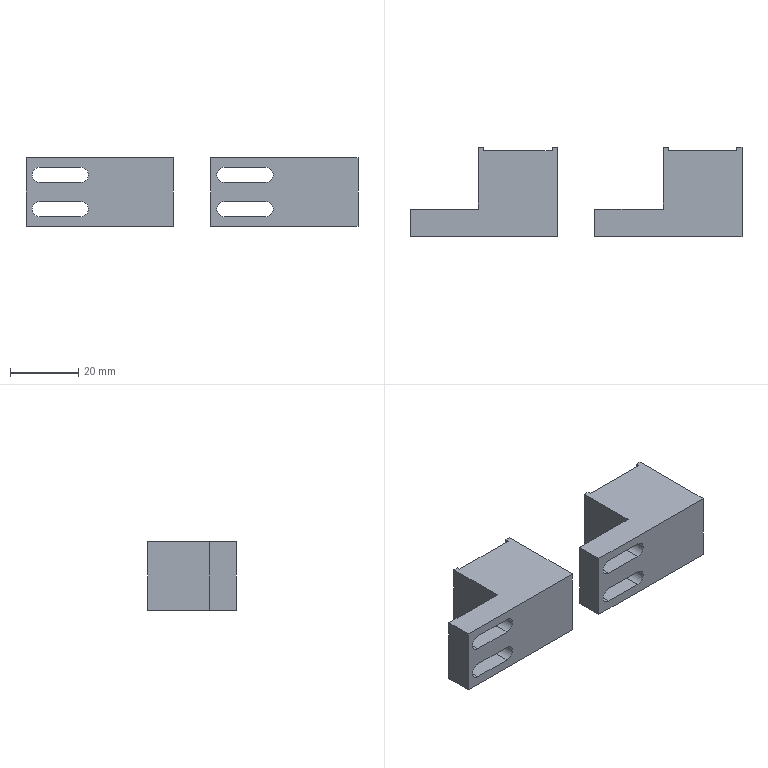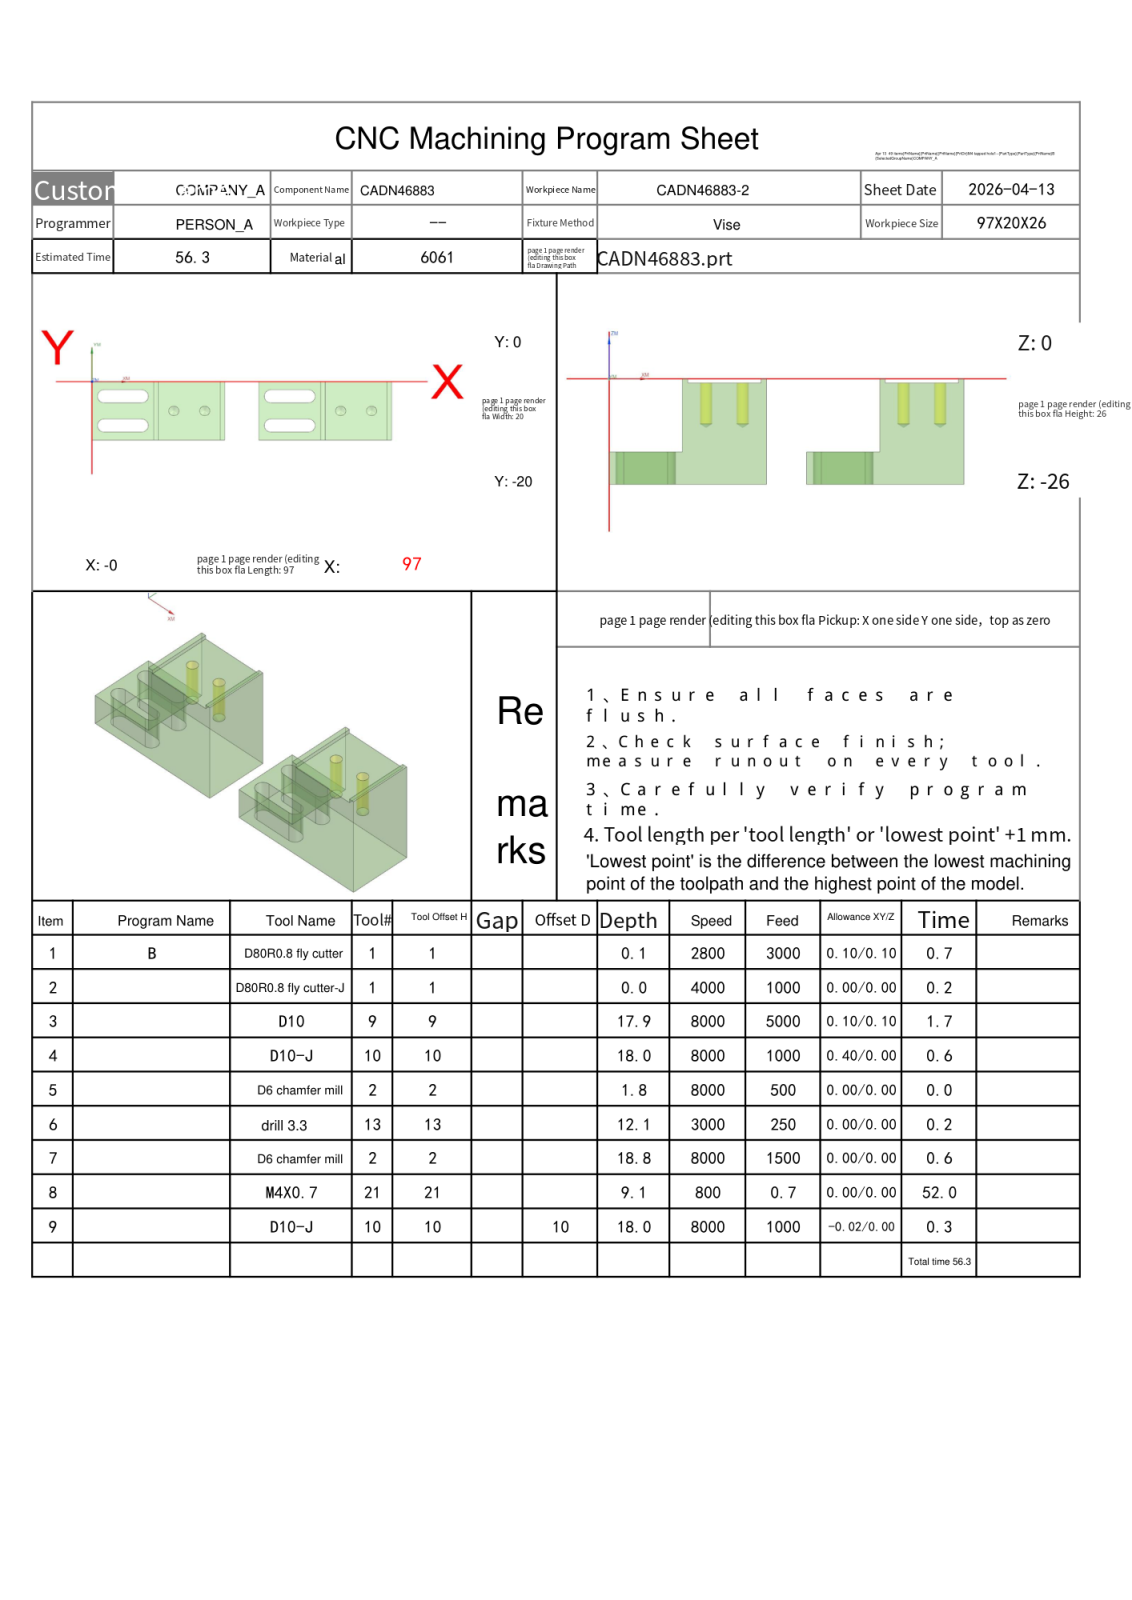NC program | NX | posted by the shop | part box 97 x 26 x 20 mm
Whole program:
%
O0001
(Machine time: 104.35 MIN)
(===Total Tool:6===)
(T1=D80R0.8 fly cutter D=80.  R=0.8  D-  H01 Z=-0.   )
(T9=D10     D=10.  R=0.   D-  H09 Z=-17.9 )
(T10=D10-J  D=10.  R=0.   D-  H10 Z=-18.  )
(T2=D6 chamfer mill   D=6.   R=0.   D-  H02 Z=-18.8 )
(T13=drill 3.3  D=3.3  DR_a=118 D-  H13 Z=-12.09)
(T21=M4X0.7 D=3.3  DR_a=180 D-  H21 Z=-9.1  )
G80 G90 G17 G49 G40
G91 G28 Z0
M01
N1 T01 M06
(D80R0.8 fly cutter  D=80. R=0.8 H=01 ce=0.10 di=0.10)
G00 G90 G54 X149.097 Y-10. M03 S2800
G43 H01 Z20.
M08
Z5.513
G01 Z3.513 F3000.
X137.097
X-40.097
X-52.097
Z5.513
G00 X149.097
Z5.025
G01 Z3.025
X137.097
X-40.097
X-52.097
Z5.025
G00 X149.097
Z4.538
G01 Z2.538
X137.097
X-40.097
X-52.097
Z4.538
G00 X149.097
Z4.05
G01 Z2.05
X137.097
X-40.097
X-52.097
Z4.05
G00 Z20.
X149.097
Z3.563
G01 Z1.563
X137.097
X-40.097
X-52.097
Z3.563
G00 Z20.
X149.097
Z3.075
G01 Z1.075
X137.097
X-40.097
X-52.097
Z3.075
G00 Z20.
X149.097
Z2.588
G01 Z.588
X137.097
X-40.097
X-52.097
Z2.588
G00 Z20.
X149.097
Z2.1
G01 Z.1
X137.097
X-40.097
X-52.097
Z2.1
G00 Z20.
G91 G28 Z0.0
M05
M09
G91 G28 Z0.0
M01
N2 T01 M06
(D80R0.8 fly cutter-J  D=80. R=0.8 H=01 ce=0.00 di=0.00)
G00 G90 G54 X148.999 Y-10. M03 S4000
G43 H01 Z20.
M08
Z2.
G01 Z0.0 F1000.
X136.999
X-39.999
X-51.999
Z2.
G00 Z20.
G91 G28 Z0.0
M05
M09
G91 G28 Z0.0
M01
N3 T09 M06
(D10  D=10. R=0. H=09 ce=0.10 di=0.10)
G00 G90 G54 X-.1 Y-28. M03 S8000
G43 H09 Z13.8
M08
Z.903
G01 Z-.597 F5000.
Y-24.9
Y3.9
G02 X.9 Y4.9 I1. J0.0
G01 X6.4
G02 X7.4 Y3.9 I0.0 J-1.
G01 Y-24.044
G03 X8.246 Y-25.032 I1. J0.0
G01 X13.746 Y-25.888
X13.9 Y-25.9
G03 X14.9 Y-24.9 I0.0 J1.
G01 Y4.9
Y8.1
Z.903
G00 X-.1 Y-28.
Z.307
G01 Z-1.193
Y-24.9
Y3.9
G02 X.9 Y4.9 I1. J0.0
G01 X6.4
G02 X7.4 Y3.9 I0.0 J-1.
G01 Y-24.044
G03 X8.246 Y-25.032 I1. J0.0
G01 X13.746 Y-25.888
X13.9 Y-25.9
G03 X14.9 Y-24.9 I0.0 J1.
G01 Y4.9
Y8.1
Z.307
G00 X-.1 Y-28.
Z-.29
G01 Z-1.79
Y-24.9
Y3.9
G02 X.9 Y4.9 I1. J0.0
G01 X6.4
G02 X7.4 Y3.9 I0.0 J-1.
G01 Y-24.044
G03 X8.246 Y-25.032 I1. J0.0
G01 X13.746 Y-25.888
X13.9 Y-25.9
G03 X14.9 Y-24.9 I0.0 J1.
G01 Y4.9
Y8.1
Z-.29
G00 X-.1 Y-28.
Z-.887
G01 Z-2.387
Y-24.9
Y3.9
G02 X.9 Y4.9 I1. J0.0
G01 X6.4
G02 X7.4 Y3.9 I0.0 J-1.
G01 Y-24.044
G03 X8.246 Y-25.032 I1. J0.0
G01 X13.746 Y-25.888
X13.9 Y-25.9
G03 X14.9 Y-24.9 I0.0 J1.
G01 Y4.9
Y8.1
Z-.887
G00 X-.1 Y-28.
Z-1.483
G01 Z-2.983
Y-24.9
Y3.9
G02 X.9 Y4.9 I1. J0.0
G01 X6.4
G02 X7.4 Y3.9 I0.0 J-1.
G01 Y-24.044
G03 X8.246 Y-25.032 I1. J0.0
G01 X13.746 Y-25.888
X13.9 Y-25.9
G03 X14.9 Y-24.9 I0.0 J1.
G01 Y4.9
Y8.1
Z-1.483
G00 X-.1 Y-28.
Z-2.08
G01 Z-3.58
Y-24.9
Y3.9
G02 X.9 Y4.9 I1. J0.0
G01 X6.4
G02 X7.4 Y3.9 I0.0 J-1.
G01 Y-24.044
G03 X8.246 Y-25.032 I1. J0.0
G01 X13.746 Y-25.888
X13.9 Y-25.9
G03 X14.9 Y-24.9 I0.0 J1.
G01 Y4.9
Y8.1
Z-2.08
G00 X-.1 Y-28.
Z-2.677
G01 Z-4.177
Y-24.9
Y3.9
G02 X.9 Y4.9 I1. J0.0
G01 X6.4
G02 X7.4 Y3.9 I0.0 J-1.
G01 Y-24.044
G03 X8.246 Y-25.032 I1. J0.0
G01 X13.746 Y-25.888
X13.9 Y-25.9
G03 X14.9 Y-24.9 I0.0 J1.
G01 Y4.9
Y8.1
Z-2.677
G00 X-.1 Y-28.
Z-3.273
G01 Z-4.773
Y-24.9
Y3.9
G02 X.9 Y4.9 I1. J0.0
G01 X6.4
G02 X7.4 Y3.9 I0.0 J-1.
G01 Y-24.044
G03 X8.246 Y-25.032 I1. J0.0
G01 X13.746 Y-25.888
X13.9 Y-25.9
G03 X14.9 Y-24.9 I0.0 J1.
G01 Y4.9
Y8.1
Z-3.273
G00 X-.1 Y-28.
Z-3.87
G01 Z-5.37
Y-24.9
Y3.9
G02 X.9 Y4.9 I1. J0.0
G01 X6.4
G02 X7.4 Y3.9 I0.0 J-1.
G01 Y-24.044
G03 X8.246 Y-25.032 I1. J0.0
G01 X13.746 Y-25.888
X13.9 Y-25.9
G03 X14.9 Y-24.9 I0.0 J1.
G01 Y4.9
Y8.1
Z-3.87
G00 X-.1 Y-28.
Z-4.467
G01 Z-5.967
Y-24.9
Y3.9
G02 X.9 Y4.9 I1. J0.0
G01 X6.4
G02 X7.4 Y3.9 I0.0 J-1.
G01 Y-24.044
G03 X8.246 Y-25.032 I1. J0.0
G01 X13.746 Y-25.888
X13.9 Y-25.9
G03 X14.9 Y-24.9 I0.0 J1.
G01 Y4.9
Y8.1
Z-4.467
G00 X-.1 Y-28.
Z-5.063
G01 Z-6.563
Y-24.9
Y3.9
G02 X.9 Y4.9 I1. J0.0
G01 X6.4
G02 X7.4 Y3.9 I0.0 J-1.
G01 Y-24.044
G03 X8.246 Y-25.032 I1. J0.0
G01 X13.746 Y-25.888
X13.9 Y-25.9
G03 X14.9 Y-24.9 I0.0 J1.
G01 Y4.9
Y8.1
Z-5.063
G00 X-.1 Y-28.
Z-5.66
G01 Z-7.16
Y-24.9
Y3.9
G02 X.9 Y4.9 I1. J0.0
G01 X6.4
G02 X7.4 Y3.9 I0.0 J-1.
G01 Y-24.044
G03 X8.246 Y-25.032 I1. J0.0
G01 X13.746 Y-25.888
X13.9 Y-25.9
G03 X14.9 Y-24.9 I0.0 J1.
G01 Y4.9
Y8.1
Z-5.66
G00 X-.1 Y-28.
Z-6.257
G01 Z-7.757
Y-24.9
Y3.9
G02 X.9 Y4.9 I1. J0.0
G01 X6.4
G02 X7.4 Y3.9 I0.0 J-1.
G01 Y-24.044
G03 X8.246 Y-25.032 I1. J0.0
G01 X13.746 Y-25.888
X13.9 Y-25.9
G03 X14.9 Y-24.9 I0.0 J1.
G01 Y4.9
Y8.1
Z-6.257
G00 X-.1 Y-28.
Z-6.853
G01 Z-8.353
Y-24.9
Y3.9
G02 X.9 Y4.9 I1. J0.0
G01 X6.4
G02 X7.4 Y3.9 I0.0 J-1.
G01 Y-24.044
G03 X8.246 Y-25.032 I1. J0.0
G01 X13.746 Y-25.888
X13.9 Y-25.9
G03 X14.9 Y-24.9 I0.0 J1.
G01 Y4.9
Y8.1
Z-6.853
G00 X-.1 Y-28.
Z-7.45
G01 Z-8.95
Y-24.9
Y3.9
G02 X.9 Y4.9 I1. J0.0
G01 X6.4
G02 X7.4 Y3.9 I0.0 J-1.
G01 Y-24.044
G03 X8.246 Y-25.032 I1. J0.0
G01 X13.746 Y-25.888
X13.9 Y-25.9
G03 X14.9 Y-24.9 I0.0 J1.
G01 Y4.9
Y8.1
Z-7.45
G00 X-.1 Y-28.
Z-8.047
G01 Z-9.547
Y-24.9
Y3.9
G02 X.9 Y4.9 I1. J0.0
G01 X6.4
G02 X7.4 Y3.9 I0.0 J-1.
G01 Y-24.044
G03 X8.246 Y-25.032 I1. J0.0
G01 X13.746 Y-25.888
X13.9 Y-25.9
G03 X14.9 Y-24.9 I0.0 J1.
G01 Y4.9
Y8.1
Z-8.047
G00 X-.1 Y-28.
Z-8.643
G01 Z-10.143
Y-24.9
Y3.9
G02 X.9 Y4.9 I1. J0.0
G01 X6.4
G02 X7.4 Y3.9 I0.0 J-1.
G01 Y-24.044
G03 X8.246 Y-25.032 I1. J0.0
G01 X13.746 Y-25.888
X13.9 Y-25.9
G03 X14.9 Y-24.9 I0.0 J1.
G01 Y4.9
Y8.1
Z-8.643
G00 X-.1 Y-28.
Z-9.24
G01 Z-10.74
Y-24.9
Y3.9
G02 X.9 Y4.9 I1. J0.0
G01 X6.4
G02 X7.4 Y3.9 I0.0 J-1.
G01 Y-24.044
G03 X8.246 Y-25.032 I1. J0.0
G01 X13.746 Y-25.888
X13.9 Y-25.9
G03 X14.9 Y-24.9 I0.0 J1.
G01 Y4.9
Y8.1
Z-9.24
G00 X-.1 Y-28.
Z-9.837
G01 Z-11.337
Y-24.9
Y3.9
G02 X.9 Y4.9 I1. J0.0
G01 X6.4
G02 X7.4 Y3.9 I0.0 J-1.
G01 Y-24.044
G03 X8.246 Y-25.032 I1. J0.0
G01 X13.746 Y-25.888
X13.9 Y-25.9
G03 X14.9 Y-24.9 I0.0 J1.
G01 Y4.9
Y8.1
Z-9.837
G00 X-.1 Y-28.
Z-10.433
G01 Z-11.933
Y-24.9
Y3.9
G02 X.9 Y4.9 I1. J0.0
G01 X6.4
G02 X7.4 Y3.9 I0.0 J-1.
G01 Y-24.044
G03 X8.246 Y-25.032 I1. J0.0
G01 X13.746 Y-25.888
X13.9 Y-25.9
G03 X14.9 Y-24.9 I0.0 J1.
G01 Y4.9
Y8.1
Z-10.433
G00 X-.1 Y-28.
Z-11.03
G01 Z-12.53
Y-24.9
Y3.9
G02 X.9 Y4.9 I1. J0.0
G01 X6.4
G02 X7.4 Y3.9 I0.0 J-1.
G01 Y-24.044
G03 X8.246 Y-25.032 I1. J0.0
G01 X13.746 Y-25.888
X13.9 Y-25.9
G03 X14.9 Y-24.9 I0.0 J1.
G01 Y4.9
Y8.1
Z-11.03
G00 X-.1 Y-28.
Z-11.627
G01 Z-13.127
Y-24.9
Y3.9
G02 X.9 Y4.9 I1. J0.0
G01 X6.4
G02 X7.4 Y3.9 I0.0 J-1.
G01 Y-24.044
G03 X8.246 Y-25.032 I1. J0.0
G01 X13.746 Y-25.888
X13.9 Y-25.9
G03 X14.9 Y-24.9 I0.0 J1.
G01 Y4.9
Y8.1
Z-11.627
G00 X-.1 Y-28.
Z-12.223
G01 Z-13.723
Y-24.9
Y3.9
G02 X.9 Y4.9 I1. J0.0
G01 X6.4
G02 X7.4 Y3.9 I0.0 J-1.
G01 Y-24.044
G03 X8.246 Y-25.032 I1. J0.0
G01 X13.746 Y-25.888
X13.9 Y-25.9
G03 X14.9 Y-24.9 I0.0 J1.
G01 Y4.9
Y8.1
Z-12.223
G00 X-.1 Y-28.
Z-12.82
G01 Z-14.32
Y-24.9
Y3.9
G02 X.9 Y4.9 I1. J0.0
G01 X6.4
G02 X7.4 Y3.9 I0.0 J-1.
G01 Y-24.044
G03 X8.246 Y-25.032 I1. J0.0
G01 X13.746 Y-25.888
X13.9 Y-25.9
G03 X14.9 Y-24.9 I0.0 J1.
G01 Y4.9
Y8.1
Z-12.82
G00 X-.1 Y-28.
Z-13.417
G01 Z-14.917
Y-24.9
Y3.9
G02 X.9 Y4.9 I1. J0.0
G01 X6.4
G02 X7.4 Y3.9 I0.0 J-1.
G01 Y-24.044
G03 X8.246 Y-25.032 I1. J0.0
G01 X13.746 Y-25.888
X13.9 Y-25.9
G03 X14.9 Y-24.9 I0.0 J1.
G01 Y4.9
Y8.1
Z-13.417
G00 X-.1 Y-28.
Z-14.013
G01 Z-15.513
Y-24.9
Y3.9
G02 X.9 Y4.9 I1. J0.0
G01 X6.4
G02 X7.4 Y3.9 I0.0 J-1.
G01 Y-24.044
G03 X8.246 Y-25.032 I1. J0.0
G01 X13.746 Y-25.888
X13.9 Y-25.9
G03 X14.9 Y-24.9 I0.0 J1.
G01 Y4.9
Y8.1
Z-14.013
G00 X-.1 Y-28.
Z-14.61
G01 Z-16.11
Y-24.9
Y3.9
G02 X.9 Y4.9 I1. J0.0
G01 X6.4
G02 X7.4 Y3.9 I0.0 J-1.
G01 Y-24.044
G03 X8.246 Y-25.032 I1. J0.0
G01 X13.746 Y-25.888
X13.9 Y-25.9
G03 X14.9 Y-24.9 I0.0 J1.
G01 Y4.9
Y8.1
Z-14.61
G00 X-.1 Y-28.
Z-15.207
G01 Z-16.707
Y-24.9
Y3.9
G02 X.9 Y4.9 I1. J0.0
G01 X6.4
G02 X7.4 Y3.9 I0.0 J-1.
G01 Y-24.044
G03 X8.246 Y-25.032 I1. J0.0
G01 X13.746 Y-25.888
X13.9 Y-25.9
G03 X14.9 Y-24.9 I0.0 J1.
G01 Y4.9
Y8.1
Z-15.207
G00 X-.1 Y-28.
Z-15.803
G01 Z-17.303
Y-24.9
Y3.9
G02 X.9 Y4.9 I1. J0.0
G01 X6.4
G02 X7.4 Y3.9 I0.0 J-1.
G01 Y-24.044
G03 X8.246 Y-25.032 I1. J0.0
G01 X13.746 Y-25.888
X13.9 Y-25.9
G03 X14.9 Y-24.9 I0.0 J1.
G01 Y4.9
Y8.1
Z-15.803
G00 X-.1 Y-28.
Z-16.4
G01 Z-17.9
Y-24.9
Y3.9
G02 X.9 Y4.9 I1. J0.0
G01 X6.4
G02 X7.4 Y3.9 I0.0 J-1.
G01 Y-24.044
G03 X8.246 Y-25.032 I1. J0.0
G01 X13.746 Y-25.888
X13.9 Y-25.9
G03 X14.9 Y-24.9 I0.0 J1.
G01 Y4.9
Y8.1
Z-16.4
G00 Z13.8
X53.9 Y-28.
Z.903
G01 Z-.597
Y-24.9
Y3.9
G02 X54.9 Y4.9 I1. J0.0
G01 X60.4
G02 X61.4 Y3.9 I0.0 J-1.
G01 Y-24.044
G03 X62.246 Y-25.032 I1. J0.0
G01 X67.746 Y-25.888
X67.9 Y-25.9
G03 X68.9 Y-24.9 I0.0 J1.
G01 Y4.9
Y8.1
Z.903
G00 X53.9 Y-28.
Z.307
G01 Z-1.193
Y-24.9
Y3.9
G02 X54.9 Y4.9 I1. J0.0
G01 X60.4
G02 X61.4 Y3.9 I0.0 J-1.
G01 Y-24.044
G03 X62.246 Y-25.032 I1. J0.0
G01 X67.746 Y-25.888
X67.9 Y-25.9
G03 X68.9 Y-24.9 I0.0 J1.
G01 Y4.9
Y8.1
Z.307
G00 X53.9 Y-28.
Z-.29
G01 Z-1.79
Y-24.9
Y3.9
G02 X54.9 Y4.9 I1. J0.0
G01 X60.4
G02 X61.4 Y3.9 I0.0 J-1.
G01 Y-24.044
G03 X62.246 Y-25.032 I1. J0.0
G01 X67.746 Y-25.888
X67.9 Y-25.9
G03 X68.9 Y-24.9 I0.0 J1.
G01 Y4.9
Y8.1
Z-.29
G00 X53.9 Y-28.
Z-.887
G01 Z-2.387
Y-24.9
Y3.9
G02 X54.9 Y4.9 I1. J0.0
G01 X60.4
G02 X61.4 Y3.9 I0.0 J-1.
G01 Y-24.044
G03 X62.246 Y-25.032 I1. J0.0
G01 X67.746 Y-25.888
X67.9 Y-25.9
G03 X68.9 Y-24.9 I0.0 J1.
G01 Y4.9
Y8.1
Z-.887
G00 X53.9 Y-28.
Z-1.483
G01 Z-2.983
Y-24.9
Y3.9
G02 X54.9 Y4.9 I1. J0.0
G01 X60.4
G02 X61.4 Y3.9 I0.0 J-1.
G01 Y-24.044
G03 X62.246 Y-25.032 I1. J0.0
G01 X67.746 Y-25.888
X67.9 Y-25.9
G03 X68.9 Y-24.9 I0.0 J1.
G01 Y4.9
Y8.1
Z-1.483
G00 X53.9 Y-28.
Z-2.08
G01 Z-3.58
Y-24.9
Y3.9
G02 X54.9 Y4.9 I1. J0.0
G01 X60.4
G02 X61.4 Y3.9 I0.0 J-1.
G01 Y-24.044
G03 X62.246 Y-25.032 I1. J0.0
G01 X67.746 Y-25.888
X67.9 Y-25.9
G03 X68.9 Y-24.9 I0.0 J1.
G01 Y4.9
Y8.1
Z-2.08
G00 X53.9 Y-28.
Z-2.677
G01 Z-4.177
Y-24.9
Y3.9
G02 X54.9 Y4.9 I1. J0.0
G01 X60.4
G02 X61.4 Y3.9 I0.0 J-1.
G01 Y-24.044
G03 X62.246 Y-25.032 I1. J0.0
G01 X67.746 Y-25.888
X67.9 Y-25.9
G03 X68.9 Y-24.9 I0.0 J1.
G01 Y4.9
Y8.1
Z-2.677
G00 X53.9 Y-28.
Z-3.273
G01 Z-4.773
Y-24.9
Y3.9
G02 X54.9 Y4.9 I1. J0.0
G01 X60.4
G02 X61.4 Y3.9 I0.0 J-1.
G01 Y-24.044
G03 X62.246 Y-25.032 I1. J0.0
G01 X67.746 Y-25.888
X67.9 Y-25.9
G03 X68.9 Y-24.9 I0.0 J1.
G01 Y4.9
Y8.1
Z-3.273
G00 X53.9 Y-28.
Z-3.87
G01 Z-5.37
Y-24.9
Y3.9
G02 X54.9 Y4.9 I1. J0.0
G01 X60.4
G02 X61.4 Y3.9 I0.0 J-1.
G01 Y-24.044
G03 X62.246 Y-25.032 I1. J0.0
G01 X67.746 Y-25.888
X67.9 Y-25.9
G03 X68.9 Y-24.9 I0.0 J1.
G01 Y4.9
Y8.1
Z-3.87
G00 X53.9 Y-28.
Z-4.467
G01 Z-5.967
Y-24.9
Y3.9
G02 X54.9 Y4.9 I1. J0.0
G01 X60.4
G02 X61.4 Y3.9 I0.0 J-1.
G01 Y-24.044
G03 X62.246 Y-25.032 I1. J0.0
G01 X67.746 Y-25.888
X67.9 Y-25.9
G03 X68.9 Y-24.9 I0.0 J1.
G01 Y4.9
Y8.1
Z-4.467
G00 X53.9 Y-28.
Z-5.063
G01 Z-6.563
Y-24.9
Y3.9
G02 X54.9 Y4.9 I1. J0.0
G01 X60.4
G02 X61.4 Y3.9 I0.0 J-1.
G01 Y-24.044
G03 X62.246 Y-25.032 I1. J0.0
G01 X67.746 Y-25.888
X67.9 Y-25.9
G03 X68.9 Y-24.9 I0.0 J1.
G01 Y4.9
Y8.1
Z-5.063
G00 X53.9 Y-28.
Z-5.66
G01 Z-7.16
Y-24.9
Y3.9
G02 X54.9 Y4.9 I1. J0.0
G01 X60.4
G02 X61.4 Y3.9 I0.0 J-1.
G01 Y-24.044
G03 X62.246 Y-25.032 I1. J0.0
G01 X67.746 Y-25.888
X67.9 Y-25.9
G03 X68.9 Y-24.9 I0.0 J1.
G01 Y4.9
Y8.1
Z-5.66
G00 X53.9 Y-28.
Z-6.257
G01 Z-7.757
Y-24.9
Y3.9
G02 X54.9 Y4.9 I1. J0.0
G01 X60.4
G02 X61.4 Y3.9 I0.0 J-1.
G01 Y-24.044
G03 X62.246 Y-25.032 I1. J0.0
G01 X67.746 Y-25.888
X67.9 Y-25.9
G03 X68.9 Y-24.9 I0.0 J1.
G01 Y4.9
Y8.1
Z-6.257
G00 X53.9 Y-28.
Z-6.853
G01 Z-8.353
Y-24.9
Y3.9
G02 X54.9 Y4.9 I1. J0.0
G01 X60.4
G02 X61.4 Y3.9 I0.0 J-1.
G01 Y-24.044
G03 X62.246 Y-25.032 I1. J0.0
G01 X67.746 Y-25.888
X67.9 Y-25.9
G03 X68.9 Y-24.9 I0.0 J1.
G01 Y4.9
Y8.1
Z-6.853
G00 X53.9 Y-28.
Z-7.45
G01 Z-8.95
Y-24.9
Y3.9
G02 X54.9 Y4.9 I1. J0.0
G01 X60.4
G02 X61.4 Y3.9 I0.0 J-1.
G01 Y-24.044
G03 X62.246 Y-25.032 I1. J0.0
G01 X67.746 Y-25.888
X67.9 Y-25.9
G03 X68.9 Y-24.9 I0.0 J1.
G01 Y4.9
Y8.1
Z-7.45
G00 X53.9 Y-28.
Z-8.047
G01 Z-9.547
Y-24.9
Y3.9
G02 X54.9 Y4.9 I1. J0.0
G01 X60.4
G02 X61.4 Y3.9 I0.0 J-1.
G01 Y-24.044
G03 X62.246 Y-25.032 I1. J0.0
G01 X67.746 Y-25.888
X67.9 Y-25.9
G03 X68.9 Y-24.9 I0.0 J1.
G01 Y4.9
Y8.1
Z-8.047
G00 X53.9 Y-28.
Z-8.643
G01 Z-10.143
Y-24.9
Y3.9
G02 X54.9 Y4.9 I1. J0.0
G01 X60.4
G02 X61.4 Y3.9 I0.0 J-1.
G01 Y-24.044
G03 X62.246 Y-25.032 I1. J0.0
G01 X67.746 Y-25.888
X67.9 Y-25.9
G03 X68.9 Y-24.9 I0.0 J1.
G01 Y4.9
Y8.1
Z-8.643
G00 X53.9 Y-28.
Z-9.24
G01 Z-10.74
Y-24.9
Y3.9
G02 X54.9 Y4.9 I1. J0.0
G01 X60.4
G02 X61.4 Y3.9 I0.0 J-1.
G01 Y-24.044
G03 X62.246 Y-25.032 I1. J0.0
G01 X67.746 Y-25.888
X67.9 Y-25.9
G03 X68.9 Y-24.9 I0.0 J1.
G01 Y4.9
Y8.1
Z-9.24
G00 X53.9 Y-28.
Z-9.837
G01 Z-11.337
Y-24.9
Y3.9
G02 X54.9 Y4.9 I1. J0.0
G01 X60.4
G02 X61.4 Y3.9 I0.0 J-1.
G01 Y-24.044
G03 X62.246 Y-25.032 I1. J0.0
G01 X67.746 Y-25.888
X67.9 Y-25.9
G03 X68.9 Y-24.9 I0.0 J1.
G01 Y4.9
Y8.1
Z-9.837
G00 X53.9 Y-28.
Z-10.433
G01 Z-11.933
Y-24.9
Y3.9
G02 X54.9 Y4.9 I1. J0.0
G01 X60.4
G02 X61.4 Y3.9 I0.0 J-1.
G01 Y-24.044
G03 X62.246 Y-25.032 I1. J0.0
G01 X67.746 Y-25.888
X67.9 Y-25.9
G03 X68.9 Y-24.9 I0.0 J1.
G01 Y4.9
Y8.1
Z-10.433
G00 X53.9 Y-28.
Z-11.03
G01 Z-12.53
Y-24.9
Y3.9
G02 X54.9 Y4.9 I1. J0.0
G01 X60.4
G02 X61.4 Y3.9 I0.0 J-1.
G01 Y-24.044
G03 X62.246 Y-25.032 I1. J0.0
G01 X67.746 Y-25.888
X67.9 Y-25.9
G03 X68.9 Y-24.9 I0.0 J1.
G01 Y4.9
Y8.1
Z-11.03
G00 X53.9 Y-28.
Z-11.627
G01 Z-13.127
Y-24.9
Y3.9
G02 X54.9 Y4.9 I1. J0.0
G01 X60.4
G02 X61.4 Y3.9 I0.0 J-1.
G01 Y-24.044
G03 X62.246 Y-25.032 I1. J0.0
G01 X67.746 Y-25.888
X67.9 Y-25.9
G03 X68.9 Y-24.9 I0.0 J1.
G01 Y4.9
Y8.1
Z-11.627
G00 X53.9 Y-28.
Z-12.223
G01 Z-13.723
Y-24.9
Y3.9
G02 X54.9 Y4.9 I1. J0.0
G01 X60.4
G02 X61.4 Y3.9 I0.0 J-1.
G01 Y-24.044
G03 X62.246 Y-25.032 I1. J0.0
G01 X67.746 Y-25.888
X67.9 Y-25.9
G03 X68.9 Y-24.9 I0.0 J1.
G01 Y4.9
Y8.1
Z-12.223
G00 X53.9 Y-28.
Z-12.82
G01 Z-14.32
Y-24.9
Y3.9
G02 X54.9 Y4.9 I1. J0.0
G01 X60.4
G02 X61.4 Y3.9 I0.0 J-1.
G01 Y-24.044
G03 X62.246 Y-25.032 I1. J0.0
G01 X67.746 Y-25.888
X67.9 Y-25.9
G03 X68.9 Y-24.9 I0.0 J1.
G01 Y4.9
Y8.1
Z-12.82
G00 X53.9 Y-28.
Z-13.417
G01 Z-14.917
Y-24.9
Y3.9
G02 X54.9 Y4.9 I1. J0.0
G01 X60.4
G02 X61.4 Y3.9 I0.0 J-1.
G01 Y-24.044
G03 X62.246 Y-25.032 I1. J0.0
G01 X67.746 Y-25.888
X67.9 Y-25.9
G03 X68.9 Y-24.9 I0.0 J1.
G01 Y4.9
Y8.1
Z-13.417
G00 X53.9 Y-28.
Z-14.013
G01 Z-15.513
Y-24.9
Y3.9
G02 X54.9 Y4.9 I1. J0.0
G01 X60.4
G02 X61.4 Y3.9 I0.0 J-1.
G01 Y-24.044
G03 X62.246 Y-25.032 I1. J0.0
G01 X67.746 Y-25.888
X67.9 Y-25.9
G03 X68.9 Y-24.9 I0.0 J1.
G01 Y4.9
Y8.1
Z-14.013
G00 X53.9 Y-28.
Z-14.61
G01 Z-16.11
Y-24.9
Y3.9
G02 X54.9 Y4.9 I1. J0.0
G01 X60.4
G02 X61.4 Y3.9 I0.0 J-1.
G01 Y-24.044
G03 X62.246 Y-25.032 I1. J0.0
G01 X67.746 Y-25.888
X67.9 Y-25.9
G03 X68.9 Y-24.9 I0.0 J1.
G01 Y4.9
Y8.1
Z-14.61
G00 X53.9 Y-28.
Z-15.207
G01 Z-16.707
Y-24.9
Y3.9
G02 X54.9 Y4.9 I1. J0.0
G01 X60.4
G02 X61.4 Y3.9 I0.0 J-1.
G01 Y-24.044
G03 X62.246 Y-25.032 I1. J0.0
G01 X67.746 Y-25.888
X67.9 Y-25.9
G03 X68.9 Y-24.9 I0.0 J1.
G01 Y4.9
Y8.1
Z-15.207
G00 X53.9 Y-28.
Z-15.803
G01 Z-17.303
Y-24.9
Y3.9
G02 X54.9 Y4.9 I1. J0.0
G01 X60.4
G02 X61.4 Y3.9 I0.0 J-1.
G01 Y-24.044
G03 X62.246 Y-25.032 I1. J0.0
G01 X67.746 Y-25.888
X67.9 Y-25.9
G03 X68.9 Y-24.9 I0.0 J1.
G01 Y4.9
Y8.1
Z-15.803
G00 X53.9 Y-28.
Z-16.4
G01 Z-17.9
Y-24.9
Y3.9
G02 X54.9 Y4.9 I1. J0.0
G01 X60.4
G02 X61.4 Y3.9 I0.0 J-1.
G01 Y-24.044
G03 X62.246 Y-25.032 I1. J0.0
G01 X67.746 Y-25.888
X67.9 Y-25.9
G03 X68.9 Y-24.9 I0.0 J1.
G01 Y4.9
Y8.1
Z-16.4
G00 Z13.8
G00 G90 X31.5 Y8. M03 S8000
Z13.8
Z1.05
G01 Z-.45 F4000.
Y4.9
X36.4
Y-24.9
X26.6
Y4.9
X28.632
G02 X29.526 Y4.347 I0.0 J-1.
G01 X31.324 Y.754
G03 X31.705 Y.344 I.894 J.448
G02 X31.9 Y.001 I-.205 J-.344
G01 Y-20.001
G02 X31.5 Y-20.4 I-.4 J.001
X31.1 Y-20.001 I0.0 J.4
G01 Y.001
G02 X31.5 Y.4 I.4 J-.001
X31.88 Y.126 I-.001 J-.4
G01 X34.727 Y1.072
Y8.1
Z1.05
G00 X31.5 Y8.
Z.6
G01 Z-.9
Y4.9
X36.4
Y-24.9
X26.6
Y4.9
X28.632
G02 X29.526 Y4.347 I0.0 J-1.
G01 X31.324 Y.754
G03 X31.705 Y.344 I.894 J.448
G02 X31.9 Y.001 I-.205 J-.344
G01 Y-20.001
G02 X31.5 Y-20.4 I-.4 J.001
X31.1 Y-20.001 I0.0 J.4
G01 Y.001
G02 X31.5 Y.4 I.4 J-.001
X31.88 Y.126 I-.001 J-.4
G01 X34.727 Y1.072
Y8.1
Z.6
G00 Z3.
X85.5 Y8.
Z1.05
G01 Z-.45
Y4.9
X90.4
Y-24.9
X80.6
Y4.9
X82.632
G02 X83.526 Y4.347 I0.0 J-1.
G01 X85.324 Y.754
G03 X85.705 Y.344 I.894 J.448
G02 X85.9 Y.001 I-.205 J-.344
G01 Y-20.001
G02 X85.5 Y-20.4 I-.4 J.001
X85.1 Y-20.001 I0.0 J.4
G01 Y.001
G02 X85.5 Y.4 I.4 J-.001
X85.88 Y.126 I-.001 J-.4
G01 X88.727 Y1.072
Y8.1
Z1.05
G00 X85.5 Y8.
Z.6
G01 Z-.9
Y4.9
X90.4
Y-24.9
X80.6
Y4.9
X82.632
G02 X83.526 Y4.347 I0.0 J-1.
G01 X85.324 Y.754
G03 X85.705 Y.344 I.894 J.448
G02 X85.9 Y.001 I-.205 J-.344
G01 Y-20.001
G02 X85.5 Y-20.4 I-.4 J.001
X85.1 Y-20.001 I0.0 J.4
G01 Y.001
G02 X85.5 Y.4 I.4 J-.001
X85.88 Y.126 I-.001 J-.4
G01 X88.727 Y1.072
Y8.1
Z.6
G00 Z13.8
G91 G28 Z0.0
M05
M09
G91 G28 Z0.0
M01
N4 T10 M06
(D10-J  D=10. R=0. H=10 ce=0.40 di=0.00)
G00 G90 G54 X-3. Y-27. M03 S8000
G43 H10 Z13.8
M08
Z-16.5
G01 Z-18. F1000.
G03 X-1. Y-25. I0.0 J2.
G01 Y4.1
G02 X-.1 Y5. I.9 J0.0
G01 X1.9
G02 X2.9 Y4. I0.0 J-1.
G01 Y-24.1
G03 X3.8 Y-25. I.9 J0.0
G01 X5.8
G03 X6.8 Y-24. I0.0 J1.
G01 Y4.1
G02 X7.7 Y5. I.9 J0.0
G01 X9.7
G02 X10.7 Y4. I0.0 J-1.
G01 Y-24.1
G03 X11.6 Y-25. I.9 J0.0
G01 X13.6
G03 X14.6 Y-24. I0.0 J1.
G01 Y5.
G03 X12.6 Y7. I-2. J0.0
G01 Z-16.5
G00 Z13.8
X51. Y-27.
Z-16.5
G01 Z-18.
G03 X53. Y-25. I0.0 J2.
G01 Y4.1
G02 X53.9 Y5. I.9 J0.0
G01 X55.9
G02 X56.9 Y4. I0.0 J-1.
G01 Y-24.1
G03 X57.8 Y-25. I.9 J0.0
G01 X59.8
G03 X60.8 Y-24. I0.0 J1.
G01 Y4.1
G02 X61.7 Y5. I.9 J0.0
G01 X63.7
G02 X64.7 Y4. I0.0 J-1.
G01 Y-24.1
G03 X65.6 Y-25. I.9 J0.0
G01 X67.6
G03 X68.6 Y-24. I0.0 J1.
G01 Y5.
G03 X66.6 Y7. I-2. J0.0
G01 Z-16.5
G00 Z13.8
G00 G90 X28.901 Y-27. M03 S8000
Z13.8
Z.5
G01 Z-1. F1000.
Y-23.
G03 X26.901 Y-25. I0.0 J-2.
G01 Y4.1
G02 X27.801 Y5. I.9 J0.0
G01 X30.5
G02 X31.5 Y4. I0.0 J-1.
G01 Y-24.1
G03 X32.4 Y-25. I.9 J0.0
G01 X35.1
G03 X36.1 Y-24. I0.0 J1.
G01 Y5.
G03 X34.1 Y7. I-2. J0.0
G01 Z.5
G00 Z3.
X82.901 Y-27.
Z.5
G01 Z-1.
Y-23.
G03 X80.901 Y-25. I0.0 J-2.
G01 Y4.1
G02 X81.801 Y5. I.9 J0.0
G01 X84.5
G02 X85.5 Y4. I0.0 J-1.
G01 Y-24.1
G03 X86.4 Y-25. I.9 J0.0
G01 X89.1
G03 X90.1 Y-24. I0.0 J1.
G01 Y5.
G03 X88.1 Y7. I-2. J0.0
G01 Z.5
G00 Z13.8
G91 G28 Z0.0
M05
M09
G91 G28 Z0.0
M01
N5 T02 M06
(D6 chamfer mill  D=6. R=0. H=02 ce=0.00 di=0.00)
G00 G90 G54 X90.5 Y-10. M03 S8000
G43 H02 Z20.
M08
G98 G81 X90.5 Y-10. Z-1.8 R0.0 F500.
X80.5
X36.5
X26.5
G80
G00 Z20.
G91 G28 Z0.0
M05
M09
G91 G28 Z0.0
M01
N6 T13 M06
(drill 3.3 D=3.3 DR_a=118 H=13)
G00 G90 G54 X90.5 Y-10. M03 S3000
G43 H13 Z20.
M08
G98 G83 X90.5 Y-10. Z-12.091 R0.0 F250. Q2.
X80.5
X36.5
X26.5
G80
G00 Z20.
G91 G28 Z0.0
M05
M09
G91 G28 Z0.0
M01
N7 T02 M06
(D6 chamfer mill  D=6. R=0. H=02 ce=0.00 di=0.00)
G00 G90 G54 X90.5 Y-10. M03 S8000
G43 H02 Z20.
M08
G98 G81 X90.5 Y-10. Z-3.2 R2. F500.
X80.5
X36.5
X26.5
G80
G00 Z20.
G00 G90 X19.173 Y-10.386 M03 S6500
Z20.
Z.572
G01 Z-.8 F1500.
G03 X19.373 Y-10.1 I-1.532 J1.286
G01 X19.403 Y-10.054
X19.4 Y-10.
Y0.0
G02 X20. Y.6 I.6 J0.0
G01 X21.5
G02 X22.1 Y0.0 I0.0 J-.6
G01 Y-20.
G02 X21.5 Y-20.6 I-.6 J0.0
G01 X20.
G02 X19.4 Y-20. I0.0 J.6
G01 Y-10.
X19.403 Y-9.946
X19.373 Y-9.9
G03 X19.173 Y-9.614 I-1.732 J-1.
G01 Z.572
G00 Z10.
X40.673 Y-10.386
Z.572
G01 Z-.8
G03 X40.873 Y-10.1 I-1.532 J1.286
G01 X40.903 Y-10.054
X40.9 Y-10.
Y0.0
G02 X41.5 Y.6 I.6 J0.0
G01 X43.
G02 X43.6 Y0.0 I0.0 J-.6
G01 Y-20.
G02 X43. Y-20.6 I-.6 J0.0
G01 X41.5
G02 X40.9 Y-20. I0.0 J.6
G01 Y-10.
X40.903 Y-9.946
X40.873 Y-9.9
G03 X40.673 Y-9.614 I-1.732 J-1.
G01 Z.572
G00 Z10.
X73.173 Y-10.386
Z.572
G01 Z-.8
G03 X73.373 Y-10.1 I-1.532 J1.286
G01 X73.403 Y-10.054
X73.4 Y-10.
Y0.0
G02 X74. Y.6 I.6 J0.0
G01 X75.5
G02 X76.1 Y0.0 I0.0 J-.6
G01 Y-20.
G02 X75.5 Y-20.6 I-.6 J0.0
G01 X74.
G02 X73.4 Y-20. I0.0 J.6
G01 Y-10.
X73.403 Y-9.946
X73.373 Y-9.9
G03 X73.173 Y-9.614 I-1.732 J-1.
G01 Z.572
G00 Z10.
X94.673 Y-10.386
Z.572
G01 Z-.8
G03 X94.873 Y-10.1 I-1.532 J1.286
G01 X94.903 Y-10.054
X94.9 Y-10.
Y0.0
G02 X95.5 Y.6 I.6 J0.0
G01 X97.
G02 X97.6 Y0.0 I0.0 J-.6
G01 Y-20.
G02 X97. Y-20.6 I-.6 J0.0
G01 X95.5
G02 X94.9 Y-20. I0.0 J.6
G01 Y-10.
X94.903 Y-9.946
X94.873 Y-9.9
G03 X94.673 Y-9.614 I-1.732 J-1.
G01 Z.572
G00 Z2.2
X93.82 Y-20.6
G01 Z-1.8
X77.18
Z2.2
G00 Z10.
Y.6
Z2.2
G01 Z-1.8
X93.82
Z2.2
G00 Z10.
X80.088 Y-10.876
Z-.279
G01 Z-1.8
G03 X80.397 Y-11.036 I1.075 J1.687
G01 X80.446 Y-11.06
X80.5 Y-11.05
G03 X81.55 Y-10. I0.0 J1.05
X80.5 Y-8.95 I-1.05 J0.0
X79.45 Y-10. I0.0 J-1.05
X80.5 Y-11.05 I1.05 J0.0
G01 X80.554 Y-11.06
X80.603 Y-11.036
G03 X80.912 Y-10.876 I-.765 J1.848
G01 Z-.279
G00 Z1.95
X90.088
Z-.279
G01 Z-1.8
G03 X90.397 Y-11.036 I1.075 J1.687
G01 X90.446 Y-11.06
X90.5 Y-11.05
G03 X91.55 Y-10. I0.0 J1.05
X90.5 Y-8.95 I-1.05 J0.0
X89.45 Y-10. I0.0 J-1.05
X90.5 Y-11.05 I1.05 J0.0
G01 X90.554 Y-11.06
X90.603 Y-11.036
G03 X90.912 Y-10.876 I-.765 J1.848
G01 Z-.279
G00 Z10.
X39.82 Y-20.6
Z2.2
G01 Z-1.8
X23.18
Z2.2
G00 Z10.
Y.6
Z2.2
G01 Z-1.8
X39.82
Z2.2
G00 Z10.
X26.088 Y-10.876
Z-.279
G01 Z-1.8
G03 X26.397 Y-11.036 I1.075 J1.687
G01 X26.446 Y-11.06
X26.5 Y-11.05
G03 X27.55 Y-10. I0.0 J1.05
X26.5 Y-8.95 I-1.05 J0.0
X25.45 Y-10. I0.0 J-1.05
X26.5 Y-11.05 I1.05 J0.0
G01 X26.554 Y-11.06
X26.603 Y-11.036
G03 X26.912 Y-10.876 I-.765 J1.848
G01 Z-.279
G00 Z1.95
X36.088
Z-.279
G01 Z-1.8
G03 X36.397 Y-11.036 I1.075 J1.687
G01 X36.446 Y-11.06
X36.5 Y-11.05
G03 X37.55 Y-10. I0.0 J1.05
X36.5 Y-8.95 I-1.05 J0.0
X35.45 Y-10. I0.0 J-1.05
X36.5 Y-11.05 I1.05 J0.0
G01 X36.554 Y-11.06
X36.603 Y-11.036
G03 X36.912 Y-10.876 I-.765 J1.848
G01 Z-.279
G00 Z10.
X16.873 Y-20.668
Z-1.798
G01 Z-18.8
X16.788 Y-20.608
X16.758 Y-20.6
X0.0
G02 X-.6 Y-20. I0.0 J.6
G01 Y0.0
G02 X0.0 Y.6 I.6 J0.0
G01 X16.758
X16.788 Y.608
X16.873 Y.668
Z-1.798
G00 Z-.05
X16.796 Y-3.666
Z-1.805
G01 Z-18.8
X16.776 Y-3.598
X16.733 Y-3.542
X16.727 Y-3.519
X16.703 Y-3.514
X16.631 Y-3.476
X16.322 Y-3.382
X16. Y-3.35
X4.
G03 X2.35 Y-5. I0.0 J-1.65
X4. Y-6.65 I1.65 J0.0
G01 X16.
X16.322 Y-6.618
X16.631 Y-6.524
X16.703 Y-6.486
X16.727 Y-6.481
X16.733 Y-6.458
X16.776 Y-6.402
X16.796 Y-6.334
Z-1.805
G00 Z-.05
Y-13.666
Z-1.805
G01 Z-18.8
X16.776 Y-13.598
X16.733 Y-13.542
X16.727 Y-13.519
X16.703 Y-13.514
X16.631 Y-13.476
X16.322 Y-13.382
X16. Y-13.35
X4.
G03 X2.35 Y-15. I0.0 J-1.65
X4. Y-16.65 I1.65 J0.0
G01 X10.
X16.
X16.322 Y-16.618
X16.631 Y-16.524
X16.703 Y-16.486
X16.727 Y-16.481
X16.733 Y-16.458
X16.776 Y-16.402
X16.796 Y-16.334
Z-1.805
G00 Z10.
X70.873 Y-20.668
Z-1.798
G01 Z-18.8
X70.788 Y-20.608
X70.758 Y-20.6
X54.
G02 X53.4 Y-20. I0.0 J.6
G01 Y0.0
G02 X54. Y.6 I.6 J0.0
G01 X70.758
X70.788 Y.608
X70.873 Y.668
Z-1.798
G00 Z-.05
X70.796 Y-3.666
Z-1.805
G01 Z-18.8
X70.776 Y-3.598
X70.733 Y-3.542
X70.727 Y-3.519
X70.703 Y-3.514
X70.631 Y-3.476
X70.322 Y-3.382
X70. Y-3.35
X58.
G03 X56.35 Y-5. I0.0 J-1.65
X58. Y-6.65 I1.65 J0.0
G01 X70.
X70.322 Y-6.618
X70.631 Y-6.524
X70.703 Y-6.486
X70.727 Y-6.481
X70.733 Y-6.458
X70.776 Y-6.402
X70.796 Y-6.334
Z-1.805
G00 Z-.05
Y-13.666
Z-1.805
G01 Z-18.8
X70.776 Y-13.598
X70.733 Y-13.542
X70.727 Y-13.519
X70.703 Y-13.514
X70.631 Y-13.476
X70.322 Y-13.382
X70. Y-13.35
X64.
X58.
G03 X56.35 Y-15. I0.0 J-1.65
X58. Y-16.65 I1.65 J0.0
G01 X70.
X70.322 Y-16.618
X70.631 Y-16.524
X70.703 Y-16.486
X70.727 Y-16.481
X70.733 Y-16.458
X70.776 Y-16.402
X70.796 Y-16.334
Z-1.805
G00 Z20.
G91 G28 Z0.0
M05
M09
G91 G28 Z0.0
M01
N8 T21 M06
(M4X0.7 D=3.3 DR_a=180 H=21)
G00 G90 G54 X90.5 Y-10. M03 S800
G43 H21 Z20.
M08
G95
G98 G84 X90.5 Y-10. Z-9.1 R0.0 F.7 Q3.
X80.5
X36.5
X26.5
G80
G94
G00 Z20.
G91 G28 Z0.0
M05
M09
G91 G28 Z0.0
M01
N9 T10 M06
(D10-J  D=10. R=0. H=10 ce=0.00 di=0.00)
G00 G90 G54 X12.801 Y-27. M03 S8000
G43 H10 Z13.8
M08
Z-17.
G01 Z-18. F1000.
G41 D10
X13.001
G03 X15. Y-25. I-.001 J2.
G01 Y5.
G03 X13. Y7. I-2. J0.0
G01 G40 X12.8
Z-17.
G00 Z13.8
X66.801 Y-27.
Z-17.
G01 Z-18.
G41 D10
X67.001
G03 X69. Y-25. I-.001 J2.
G01 Y5.
G03 X67.001 Y7. I-2. J0.0
G01 G40 X66.801
Z-17.
G00 Z13.8
G00 G90 X34.604 Y-27.008 M03 S8000
Z13.8
Z0.0
G01 Z-1. F1000.
G41 D10
X34.802 Y-26.98
G03 X36.52 Y-25. I-.282 J1.98
G01 Y5.
G03 X34.802 Y6.98 I-2. J0.0
G01 G40 X34.604 Y7.008
X28.396
G41 D10
X28.198 Y6.98
G03 X26.48 Y5. I.282 J-1.98
G01 Y-25.
G03 X28.198 Y-26.98 I2. J0.0
G01 G40 X28.396 Y-27.008
Z0.0
G00 Z13.8
X82.396 Y7.008
Z0.0
G01 Z-1.
G41 D10
X82.198 Y6.98
G03 X80.48 Y5. I.282 J-1.98
G01 Y-25.
G03 X82.198 Y-26.98 I2. J0.0
G01 G40 X82.396 Y-27.008
X88.604
G41 D10
X88.802 Y-26.98
G03 X90.52 Y-25. I-.282 J1.98
G01 Y5.
G03 X88.802 Y6.98 I-2. J0.0
G01 G40 X88.604 Y7.008
Z0.0
G00 Z13.8
M05
M09
G91 G28 Z0.0
G91 G28 Y0.0
M30
%